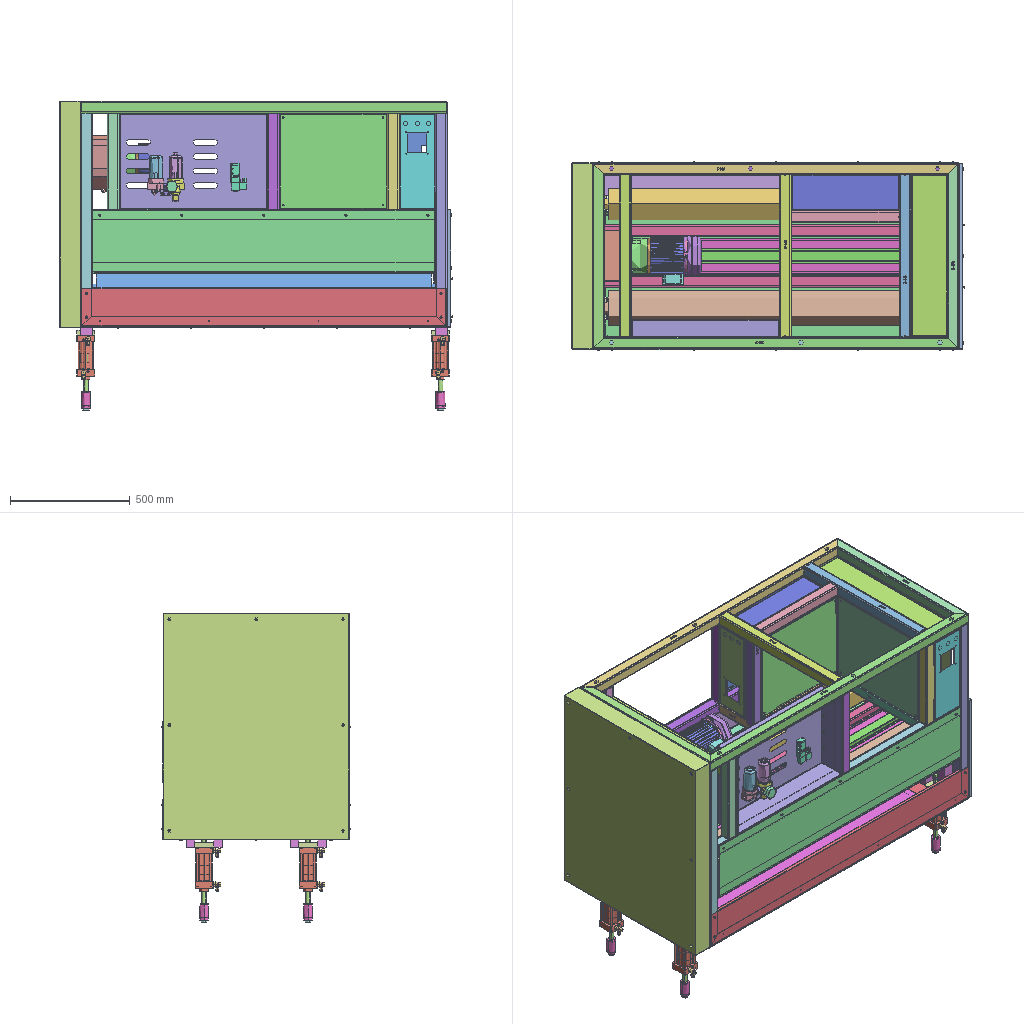Assembly | SolidWorks | 119 different items | 378 placed | box 1638 x 789 x 1291 mm
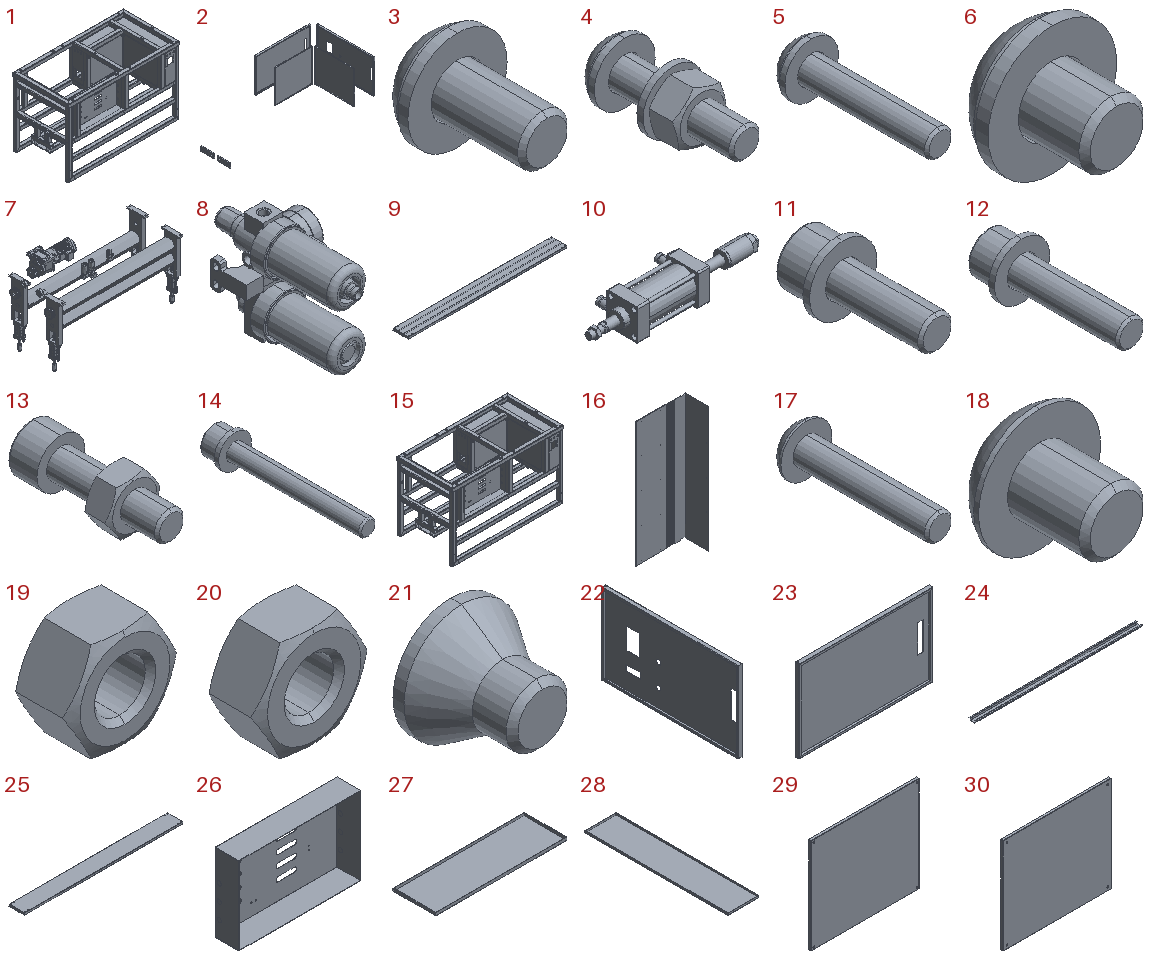Parts list (item | name | quantity | parent item | size | volume | features):
1 | (subassembly) | x1 | in 15 | - | 19240717 mm3 | -
2 | (subassembly) | x1 | in 15 | 1542 x 724.002 x 448 mm | 1639725 mm3 | -
3 | (subassembly) | x16 | - | 10 x 12.75 x 10 mm | 377.531 mm3 | -
4 | (subassembly) | x12 | - | 10 x 23.75 x 10 mm | 840.572 mm3 | -
5 | (subassembly) | x7 | - | 10 x 27.75 x 10 mm | 672.055 mm3 | -
6 | (subassembly) | x2 | - | 10 x 8.75 x 10 mm | 298.991 mm3 | -
7 | (subassembly) | x1 | - | - | 980797146154168884946852313429228984824106233416722874278836734645215409165302339514138724197191222539980428161043675585091870182479337387475146593540243456 mm3 | -
8 | (subassembly) | x1 | in 7 | 103 x 201.6 x 154 mm | 430309 mm3 | -
9 | (subassembly) | x1 | - | 1530 x 150 x 22 mm | 923330 mm3 | -
10 | (subassembly) | x4 | in 7 | 397 x 107 x 75 mm | 672153 mm3 | -
11 | (subassembly) | x4 | - | 20 x 40 x 20 mm | 4524 mm3 | -
12 | (subassembly) | x12 | - | 24 x 62 x 24 mm | 8955 mm3 | -
13 | (subassembly) | x4 | - | 11.489 x 29 x 10.527 mm | 1391 mm3 | -
14 | (subassembly) | x4 | - | 12 x 56 x 12 mm | 1944 mm3 | -
15 | (subassembly) | x1 | - | - | 20880442 mm3 | -
16 | - | x1 | - | 575.794 x 268 x 1427 mm | 3365860 mm3 | features BaseBody 1
17 | - | x7 | in 5 | 9.5 x 27.75 x 9.5 mm | 615.577 mm3 | features BaseBody 1
18 | - | x2 | in 6 | 9.5 x 8.75 x 9.5 mm | 242.513 mm3 | features BaseBody 1
19 | - | x12 | in 4 | 9.238 x 4.7 x 8 mm | 190.578 mm3 | features BaseBody 1
20 | - | x4 | in 13 | 11.547 x 5.2 x 10 mm | 340.003 mm3 | features BaseBody 1
21 | - | x10 | - | 7.53 x 6 x 7.53 mm | 127.383 mm3 | features BaseBody 1
22 | - | x1 | in 2 | 20 x 671 x 396 mm | 462181 mm3 | features BaseBody 1
23 | - | x1 | in 2 | 645 x 20 x 396 mm | 458573 mm3 | features BaseBody 1
24 | - | x1 | in 9 | 1507 x 64 x 20 mm | 295191 mm3 | features BaseBody 1
25 | - | x1 | in 9 | 1530 x 150 x 20 mm | 628139 mm3 | features BaseBody 9
26 | - | x1 | in 1 | 615 x 120 x 396 mm | 920758 mm3 | features BaseBody 1
27 | - | x2 | in 1 | 446 x 146 x 10 mm | 111927 mm3 | features BaseBody 1
28 | - | x2 | in 1 | 146 x 672 x 10 mm | 166908 mm3 | features BaseBody 1
29 | - | x1 | in 2 | 436 x 10 x 386 mm | 272050 mm3 | features BaseBody 1
30 | - | x1 | in 1 | 446 x 20 x 396 mm | 287469 mm3 | features BaseBody 5
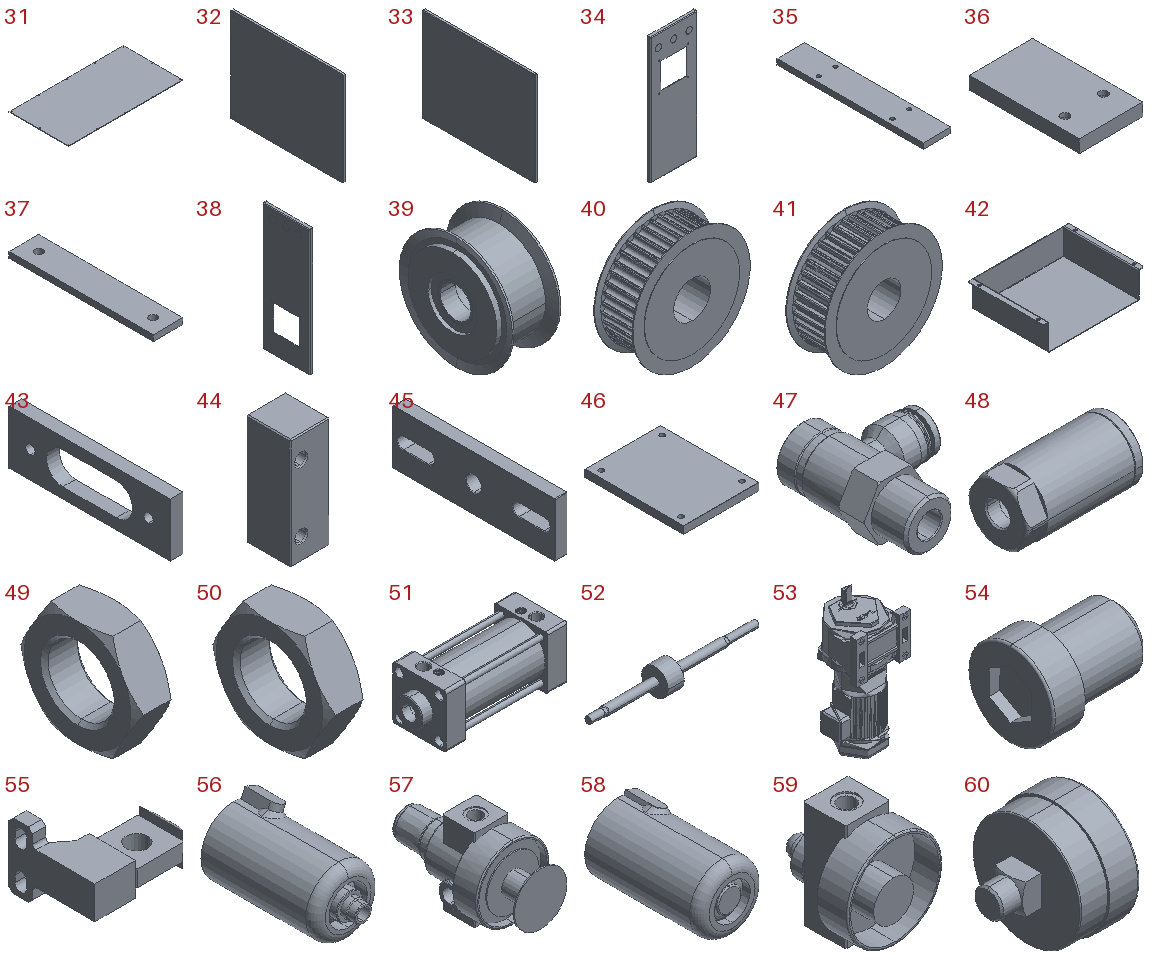31 | - | x1 | - | 1250 x 650 x 5 mm | 4061075 mm3 | features BaseBody 1
32 | - | x1 | in 1 | 20 x 472 x 396 mm | 303544 mm3 | features BaseBody 5
33 | - | x1 | in 2 | 10 x 462 x 386 mm | 287636 mm3 | features BaseBody 1
34 | - | x1 | in 1 | 146 x 10 x 396 mm | 89690 mm3 | features BaseBody 1
35 | - | x1 | in 1 | 50 x 262 x 10 mm | 127977 mm3 | features BaseBody 1
36 | - | x2 | in 1 | 50 x 86 x 10 mm | 41489 mm3 | features BaseBody 1
37 | - | x4 | in 1 | 50 x 242 x 10 mm | 118345 mm3 | features BaseBody 1
38 | - | x1 | in 1 | 10 x 146 x 396 mm | 89676 mm3 | features BaseBody 1
39 | - | x2 | in 7 | 36 x 73.9 x 73.9 mm | 85906 mm3 | features BaseBody 1
40 | - | x2 | in 7 | 111 x 38 x 111 mm | 247704 mm3 | features BaseBody 1
41 | - | x1 | in 7 | 110.9 x 38 x 110.9 mm | 257710 mm3 | features BaseBody 1
42 | - | x1 | - | 274 x 206.5 x 71.5 mm | 153067 mm3 | features BaseBody 5
43 | - | x2 | in 1 | 12 x 150 x 50 mm | 62156 mm3 | features BaseBody 1
44 | - | x2 | in 1 | 18 x 20 x 50 mm | 17163 mm3 | features BaseBody 1
45 | - | x2 | in 2 | 12 x 150 x 50 mm | 79643 mm3 | features BaseBody 1
46 | - | x1 | in 1 | 161 x 210 x 16 mm | 535538 mm3 | features BaseBody 1
47 | - | x8 | in 10 | 37.97 x 44 x 19 mm | 11551 mm3 | features BaseBody 1
48 | - | x4 | in 10 | 71 x 38 x 38 mm | 56473 mm3 | features BaseBody 1
49 | - | x4 | in 10 | 8 x 26.558 x 23 mm | 2309 mm3 | features BaseBody 1
50 | - | x4 | in 10 | 8 x 26.558 x 23 mm | 2309 mm3 | features BaseBody 1
51 | - | x4 | in 10 | 201 x 75 x 75 mm | 371064 mm3 | features BaseBody 1
52 | - | x4 | in 10 | 397 x 62.5 x 62.5 mm | 216895 mm3 | features BaseBody 1
53 | - | x1 | in 7 | - | - | features RefSurface 34, BaseBody 5
54 | - | x1 | in 8 | 10 x 8 x 8 mm | 331.342 mm3 | features BaseBody 1
55 | - | x1 | in 8 | 60 x 52.5 x 40 mm | 28461 mm3 | features BaseBody 1
56 | - | x1 | in 8 | 54.5 x 108.1 x 61.848 mm | 45492 mm3 | features BaseBody 1
57 | - | x1 | in 8 | 64 x 117.8 x 72 mm | 166401 mm3 | features BaseBody 1
58 | - | x1 | in 8 | 54.5 x 95.3 x 57.228 mm | 39263 mm3 | features BaseBody 1
59 | - | x1 | in 8 | 64 x 69.6 x 72 mm | 94903 mm3 | features BaseBody 1
60 | - | x1 | in 8 | 44.5 x 52 x 52 mm | 55458 mm3 | features BaseBody 1
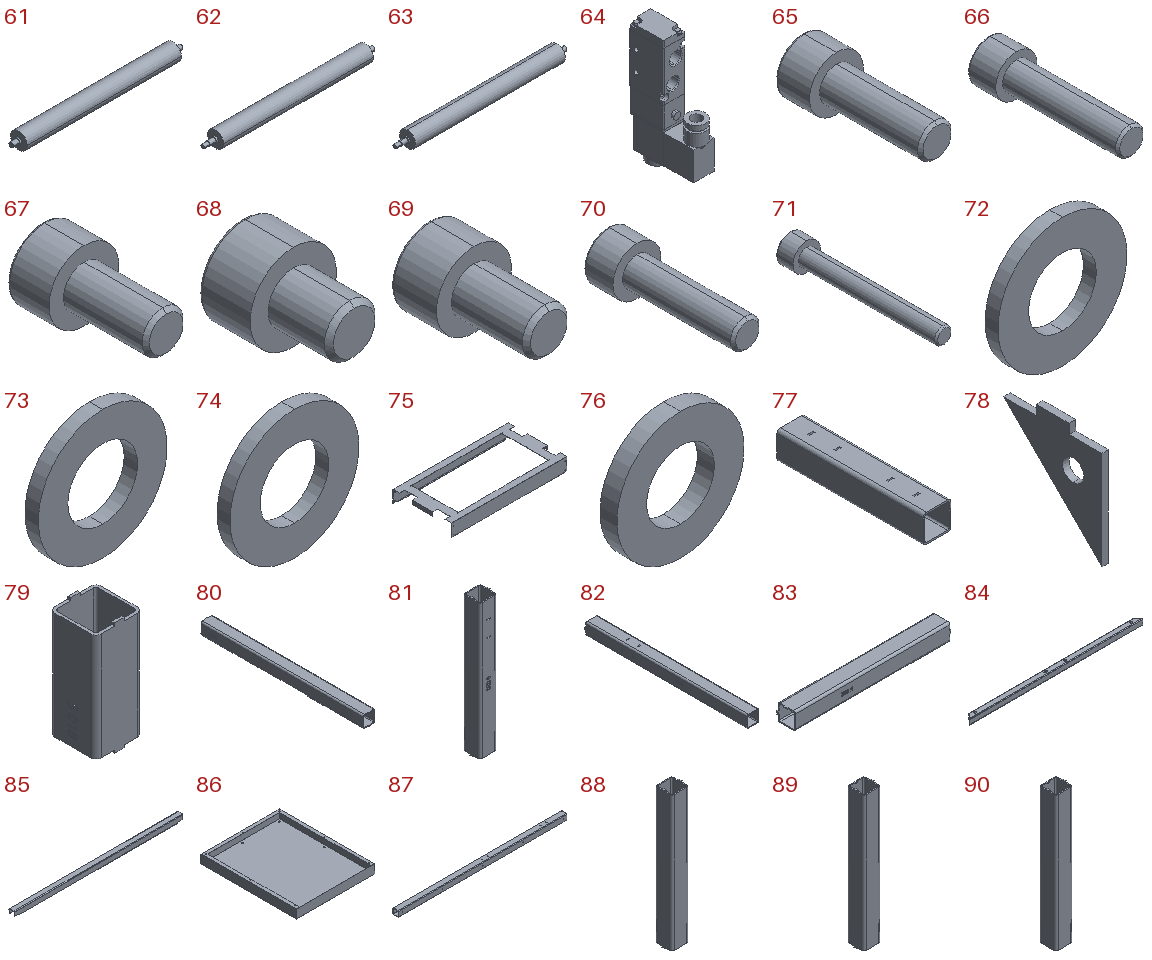61 | - | x2 | in 7 | 1540 x 150 x 150 mm | 24937177 mm3 | features BaseBody 1
62 | - | x1 | - | 1590 x 150 x 150 mm | 24977389 mm3 | features BaseBody 1
63 | - | x1 | in 7 | 1590 x 150 x 150 mm | 24977389 mm3 | features BaseBody 1
64 | - | x1 | in 7 | 22 x 66.8 x 117.8 mm | 99951 mm3 | features BaseBody 1
65 | - | x4 | in 11 | 16 x 40 x 16 mm | 4068 mm3 | features BaseBody 1
66 | - | x12 | in 12 | 18 x 62 x 18 mm | 8155 mm3 | features BaseBody 1
67 | - | x7 | - | 8.5 x 15 x 8.5 mm | 442.746 mm3 | features BaseBody 1
68 | - | x4 | - | 8.5 x 11 x 8.5 mm | 364.206 mm3 | features BaseBody 1
69 | - | x4 | - | 10 x 16 x 10 mm | 683.613 mm3 | features BaseBody 1
70 | - | x4 | in 13 | 10 x 29 x 10 mm | 1051 mm3 | features BaseBody 1
71 | - | x4 | in 14 | 10 x 56 x 10 mm | 1815 mm3 | features BaseBody 1
72 | - | x4 | in 11 | 20 x 2 x 20 mm | 455.138 mm3 | features BaseBody 1
73 | - | x12 | in 12 | 24 x 2.5 x 24 mm | 799.143 mm3 | features BaseBody 1
74 | - | x49 | in 3, 4, 5, 6 | 10 x 1 x 10 mm | 56.478 mm3 | features BaseBody 1
75 | - | x1 | - | 1528 x 781 x 165 mm | 1922839 mm3 | features BaseBody 1
76 | - | x4 | in 14 | 12 x 1.6 x 12 mm | 129.484 mm3 | features BaseBody 1
77 | - | x2 | in 1 | 50 x 262 x 50 mm | 141281 mm3 | features BaseBody 1
78 | - | x4 | in 1 | 2 x 30 x 33 mm | 893.634 mm3 | features BaseBody 1
79 | - | x2 | in 1 | 50 x 50 x 121 mm | 62514 mm3 | features BaseBody 1
80 | - | x1 | in 1 | 50 x 682 x 50 mm | 333028 mm3 | features BaseBody 1
81 | - | x1 | in 1 | 50 x 50 x 406 mm | 216470 mm3 | features BaseBody 1
82 | - | x1 | in 1 | 50 x 679 x 50 mm | 365362 mm3 | features BaseBody 1
83 | - | x1 | in 1 | 456 x 50 x 50 mm | 243710 mm3 | features BaseBody 1
84 | - | x1 | in 1 | 1527 x 50 x 50 mm | 794723 mm3 | features BaseBody 1
85 | - | x2 | in 1 | 1530 x 50 x 50 mm | 809268 mm3 | features BaseBody 1
86 | - | x1 | - | 776 x 944 x 86.5 mm | 1648928 mm3 | features BaseBody 1
87 | - | x1 | in 1 | 1436 x 50 x 50 mm | 773039 mm3 | features BaseBody 1
88 | - | x1 | in 1 | 50 x 50 x 406 mm | 216517 mm3 | features BaseBody 1
89 | - | x2 | in 1 | 50 x 50 x 406 mm | 216517 mm3 | features BaseBody 1
90 | - | x1 | in 1 | 50 x 50 x 403 mm | 216139 mm3 | features BaseBody 1
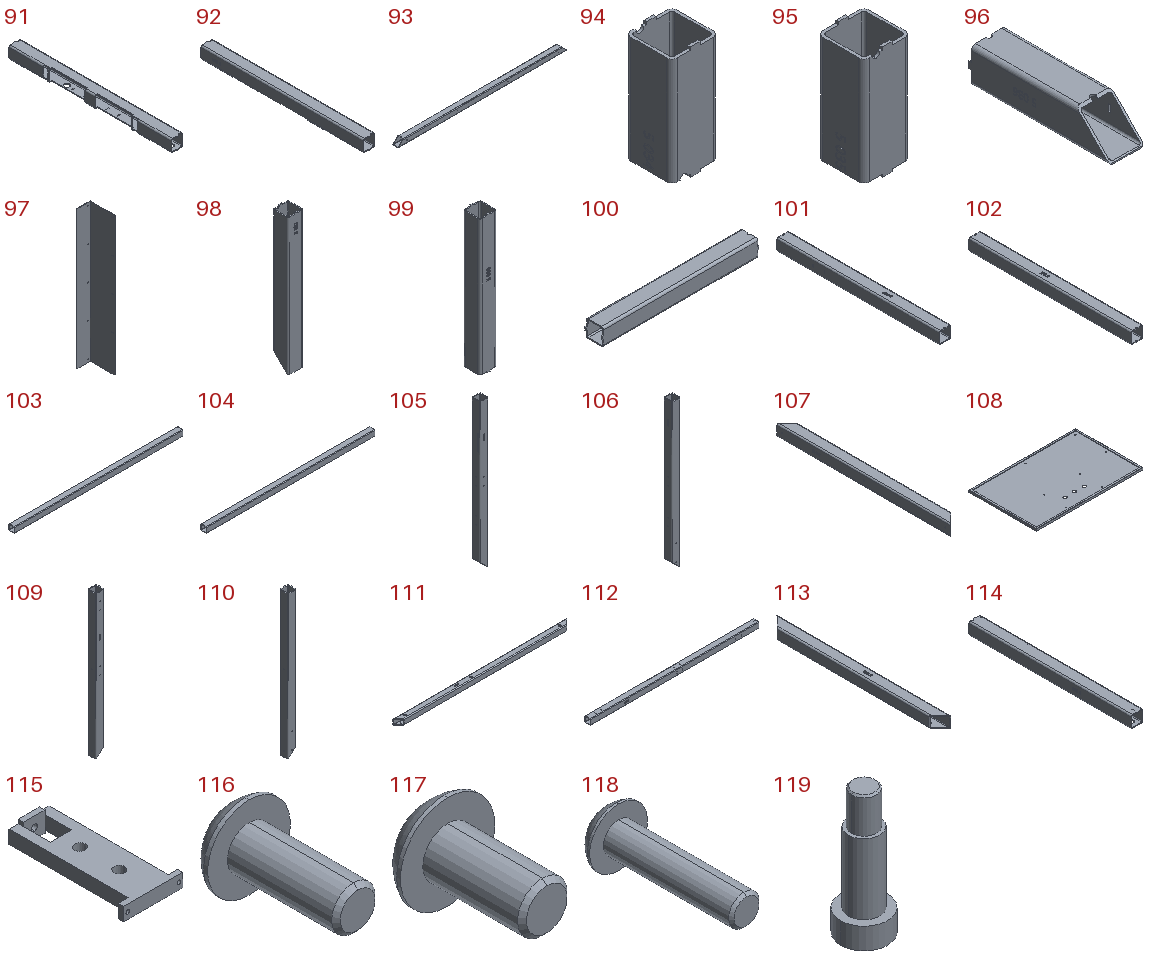91 | - | x1 | in 1 | 50 x 682 x 50 mm | 298312 mm3 | features BaseBody 1
92 | - | x1 | in 1 | 50 x 682 x 50 mm | 332876 mm3 | features BaseBody 1
93 | - | x2 | in 1 | 1527 x 50 x 50 mm | 799751 mm3 | features BaseBody 1
94 | - | x1 | in 1 | 50 x 50 x 121 mm | 62383 mm3 | features BaseBody 1
95 | - | x1 | in 1 | 50 x 50 x 121 mm | 62384 mm3 | features BaseBody 1
96 | - | x1 | in 1 | 50 x 201.5 x 50 mm | 94471 mm3 | features BaseBody 1
97 | - | x1 | - | 138.931 x 257 x 1427 mm | 1121398 mm3 | features BaseBody 1
98 | - | x1 | in 1 | 50 x 50 x 451.5 mm | 229789 mm3 | features BaseBody 1
99 | - | x1 | in 1 | 50 x 50 x 406 mm | 216667 mm3 | features BaseBody 1
100 | - | x1 | in 1 | 456 x 50 x 50 mm | 243558 mm3 | features BaseBody 1
101 | - | x1 | in 1 | 50 x 676 x 50 mm | 365028 mm3 | features BaseBody 1
102 | - | x1 | in 1 | 50 x 676 x 50 mm | 364880 mm3 | features BaseBody 1
103 | - | x1 | in 1 | 1436 x 50 x 50 mm | 773565 mm3 | features BaseBody 1
104 | - | x1 | in 1 | 1436 x 50 x 50 mm | 773588 mm3 | features BaseBody 1
105 | - | x1 | in 1 | 50 x 50 x 893.5 mm | 465694 mm3 | features BaseBody 1
106 | - | x1 | in 1 | 50 x 50 x 893.5 mm | 465622 mm3 | features BaseBody 1
107 | - | x1 | in 1 | 50 x 773 x 50 mm | 392198 mm3 | features BaseBody 1
108 | - | x1 | - | 776 x 492 x 16.5 mm | 663025 mm3 | features BaseBody 1
109 | - | x1 | in 1 | 50 x 50 x 893.5 mm | 467939 mm3 | features BaseBody 1
110 | - | x1 | in 1 | 50 x 50 x 893.5 mm | 467855 mm3 | features BaseBody 1
111 | - | x1 | in 1 | 1527 x 50 x 50 mm | 791850 mm3 | features BaseBody 1
112 | - | x1 | in 1 | 1436 x 50 x 50 mm | 769827 mm3 | features BaseBody 1
113 | - | x1 | in 1 | 50 x 773 x 50 mm | 392292 mm3 | features BaseBody 1
114 | - | x1 | in 1 | 50 x 682 x 50 mm | 361396 mm3 | features BaseBody 1
115 | - | x4 | in 7 | 222 x 466.001 x 75 mm | 3067581 mm3 | features BaseBody 2
116 | - | x5 | - | 7.6 x 12.2 x 7.6 mm | 189.389 mm3 | features BaseBody 1
117 | - | x16 | in 3 | 9.5 x 12.75 x 9.5 mm | 321.053 mm3 | features BaseBody 1
118 | - | x12 | in 4 | 9.5 x 23.75 x 9.5 mm | 537.038 mm3 | features BaseBody 1
119 | - | x2 | in 7 | 30 x 30 x 81.15 mm | 28332 mm3 | features BaseBody 1